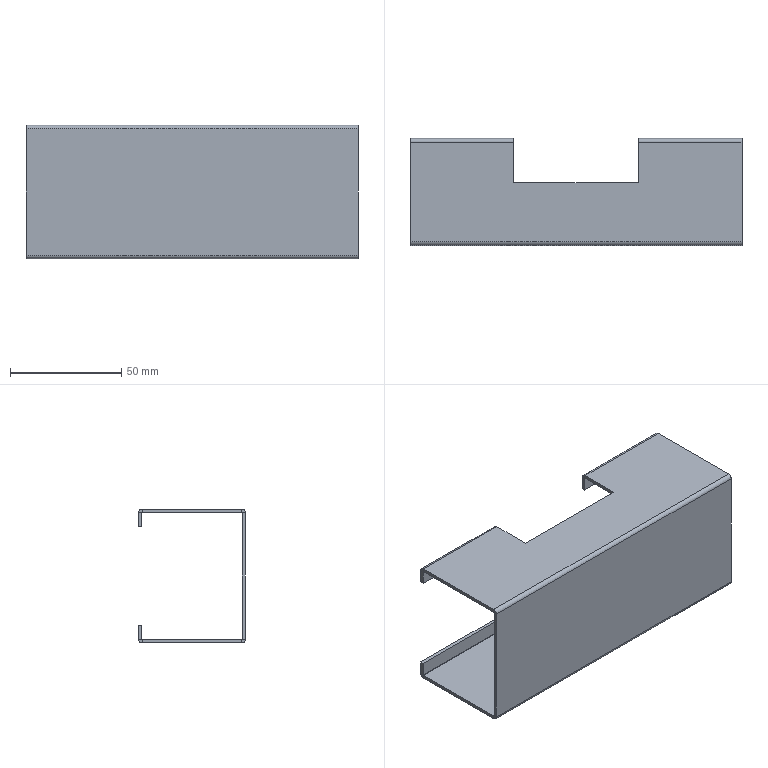Part | 1 solid | 62 faces | box 149 x 48 x 60 mm | volume 32353 mm3 | plane 50 | cylinder 12 | commonest cylinder face diameters 0.4 x6 3.4 x6
STEP:
#1=CARTESIAN_POINT('',(-28.,48.,28.3));
#2=VERTEX_POINT('',#1);
#3=CARTESIAN_POINT('',(-28.,48.,22.));
#4=VERTEX_POINT('',#3);
#5=CARTESIAN_POINT('',(-28.,48.,22.));
#6=DIRECTION('',(0.,0.,-1.));
#7=VECTOR('',#6,1000.);
#8=LINE('',#5,#7);
#9=EDGE_CURVE('',#2,#4,#8,.T.);
#10=ORIENTED_EDGE('',*,*,#9,.F.);
#11=CARTESIAN_POINT('',(-28.,46.5,28.3));
#12=VERTEX_POINT('',#11);
#13=CARTESIAN_POINT('',(-28.,48.,28.3));
#14=DIRECTION('',(0.,-1.,0.));
#15=VECTOR('',#14,1000.);
#16=LINE('',#13,#15);
#17=EDGE_CURVE('',#2,#12,#16,.T.);
#18=ORIENTED_EDGE('',*,*,#17,.T.);
#19=CARTESIAN_POINT('',(-28.,46.5,22.));
#20=VERTEX_POINT('',#19);
#21=CARTESIAN_POINT('',(-28.,46.5,22.));
#22=DIRECTION('',(0.,0.,-1.));
#23=VECTOR('',#22,1000.);
#24=LINE('',#21,#23);
#25=EDGE_CURVE('',#12,#20,#24,.T.);
#26=ORIENTED_EDGE('',*,*,#25,.T.);
#27=CARTESIAN_POINT('',(-28.,48.,22.));
#28=DIRECTION('',(0.,1.,0.));
#29=VECTOR('',#28,1000.);
#30=LINE('',#27,#29);
#31=EDGE_CURVE('',#20,#4,#30,.T.);
#32=ORIENTED_EDGE('',*,*,#31,.T.);
#33=EDGE_LOOP('',(#10,#18,#26,#32));
#34=FACE_OUTER_BOUND('',#33,.T.);
#35=CARTESIAN_POINT('',(-28.,68.,-30.));
#36=DIRECTION('',(-1.,0.,0.));
#37=DIRECTION('',(0.,0.,1.));
#38=AXIS2_PLACEMENT_3D('',#35,#36,#37);
#39=PLANE('',#38);
#40=ADVANCED_FACE('',(#34),#39,.F.);
#41=CARTESIAN_POINT('',(-28.,28.,28.5));
#42=VERTEX_POINT('',#41);
#43=CARTESIAN_POINT('',(-28.,46.3,28.5));
#44=VERTEX_POINT('',#43);
#45=CARTESIAN_POINT('',(-28.,48.,28.5));
#46=DIRECTION('',(0.,1.,0.));
#47=VECTOR('',#46,1000.);
#48=LINE('',#45,#47);
#49=EDGE_CURVE('',#42,#44,#48,.T.);
#50=ORIENTED_EDGE('',*,*,#49,.T.);
#51=CARTESIAN_POINT('',(-28.,46.3,30.));
#52=VERTEX_POINT('',#51);
#53=CARTESIAN_POINT('',(-28.,46.3,28.5));
#54=DIRECTION('',(0.,0.,1.));
#55=VECTOR('',#54,1000.);
#56=LINE('',#53,#55);
#57=EDGE_CURVE('',#44,#52,#56,.T.);
#58=ORIENTED_EDGE('',*,*,#57,.T.);
#59=CARTESIAN_POINT('',(-28.,28.,30.));
#60=VERTEX_POINT('',#59);
#61=CARTESIAN_POINT('',(-28.,48.,30.));
#62=DIRECTION('',(0.,1.,0.));
#63=VECTOR('',#62,1000.);
#64=LINE('',#61,#63);
#65=EDGE_CURVE('',#60,#52,#64,.T.);
#66=ORIENTED_EDGE('',*,*,#65,.F.);
#67=CARTESIAN_POINT('',(-28.,28.,-30.));
#68=DIRECTION('',(0.,0.,1.));
#69=VECTOR('',#68,1000.);
#70=LINE('',#67,#69);
#71=EDGE_CURVE('',#42,#60,#70,.T.);
#72=ORIENTED_EDGE('',*,*,#71,.F.);
#73=EDGE_LOOP('',(#50,#58,#66,#72));
#74=FACE_OUTER_BOUND('',#73,.T.);
#75=CARTESIAN_POINT('',(-28.,68.,-30.));
#76=DIRECTION('',(-1.,0.,0.));
#77=DIRECTION('',(0.,0.,1.));
#78=AXIS2_PLACEMENT_3D('',#75,#76,#77);
#79=PLANE('',#78);
#80=ADVANCED_FACE('',(#74),#79,.F.);
#81=CARTESIAN_POINT('',(28.,46.5,22.));
#82=VERTEX_POINT('',#81);
#83=CARTESIAN_POINT('',(28.,46.5,28.3));
#84=VERTEX_POINT('',#83);
#85=CARTESIAN_POINT('',(28.,46.5,22.));
#86=DIRECTION('',(0.,0.,1.));
#87=VECTOR('',#86,1000.);
#88=LINE('',#85,#87);
#89=EDGE_CURVE('',#82,#84,#88,.T.);
#90=ORIENTED_EDGE('',*,*,#89,.T.);
#91=CARTESIAN_POINT('',(28.,48.,28.3));
#92=VERTEX_POINT('',#91);
#93=CARTESIAN_POINT('',(28.,46.5,28.3));
#94=DIRECTION('',(0.,1.,0.));
#95=VECTOR('',#94,1000.);
#96=LINE('',#93,#95);
#97=EDGE_CURVE('',#84,#92,#96,.T.);
#98=ORIENTED_EDGE('',*,*,#97,.T.);
#99=CARTESIAN_POINT('',(28.,48.,22.));
#100=VERTEX_POINT('',#99);
#101=CARTESIAN_POINT('',(28.,48.,22.));
#102=DIRECTION('',(0.,0.,1.));
#103=VECTOR('',#102,1000.);
#104=LINE('',#101,#103);
#105=EDGE_CURVE('',#100,#92,#104,.T.);
#106=ORIENTED_EDGE('',*,*,#105,.F.);
#107=CARTESIAN_POINT('',(28.,48.,22.));
#108=DIRECTION('',(0.,-1.,0.));
#109=VECTOR('',#108,1000.);
#110=LINE('',#107,#109);
#111=EDGE_CURVE('',#100,#82,#110,.T.);
#112=ORIENTED_EDGE('',*,*,#111,.T.);
#113=EDGE_LOOP('',(#90,#98,#106,#112));
#114=FACE_OUTER_BOUND('',#113,.T.);
#115=CARTESIAN_POINT('',(28.,68.,-30.));
#116=DIRECTION('',(1.,0.,0.));
#117=DIRECTION('',(0.,0.,-1.));
#118=AXIS2_PLACEMENT_3D('',#115,#116,#117);
#119=PLANE('',#118);
#120=ADVANCED_FACE('',(#114),#119,.F.);
#121=CARTESIAN_POINT('',(28.,46.3,30.));
#122=VERTEX_POINT('',#121);
#123=CARTESIAN_POINT('',(28.,28.,30.));
#124=VERTEX_POINT('',#123);
#125=CARTESIAN_POINT('',(28.,48.,30.));
#126=DIRECTION('',(0.,-1.,0.));
#127=VECTOR('',#126,1000.);
#128=LINE('',#125,#127);
#129=EDGE_CURVE('',#122,#124,#128,.T.);
#130=ORIENTED_EDGE('',*,*,#129,.F.);
#131=CARTESIAN_POINT('',(28.,46.3,28.5));
#132=VERTEX_POINT('',#131);
#133=CARTESIAN_POINT('',(28.,46.3,30.));
#134=DIRECTION('',(0.,0.,-1.));
#135=VECTOR('',#134,1000.);
#136=LINE('',#133,#135);
#137=EDGE_CURVE('',#122,#132,#136,.T.);
#138=ORIENTED_EDGE('',*,*,#137,.T.);
#139=CARTESIAN_POINT('',(28.,28.,28.5));
#140=VERTEX_POINT('',#139);
#141=CARTESIAN_POINT('',(28.,48.,28.5));
#142=DIRECTION('',(0.,-1.,0.));
#143=VECTOR('',#142,1000.);
#144=LINE('',#141,#143);
#145=EDGE_CURVE('',#132,#140,#144,.T.);
#146=ORIENTED_EDGE('',*,*,#145,.T.);
#147=CARTESIAN_POINT('',(28.,28.,-30.));
#148=DIRECTION('',(0.,0.,1.));
#149=VECTOR('',#148,1000.);
#150=LINE('',#147,#149);
#151=EDGE_CURVE('',#140,#124,#150,.T.);
#152=ORIENTED_EDGE('',*,*,#151,.T.);
#153=EDGE_LOOP('',(#130,#138,#146,#152));
#154=FACE_OUTER_BOUND('',#153,.T.);
#155=CARTESIAN_POINT('',(28.,68.,-30.));
#156=DIRECTION('',(1.,0.,0.));
#157=DIRECTION('',(0.,0.,-1.));
#158=AXIS2_PLACEMENT_3D('',#155,#156,#157);
#159=PLANE('',#158);
#160=ADVANCED_FACE('',(#154),#159,.F.);
#161=CARTESIAN_POINT('',(-28.,46.5,-22.));
#162=VERTEX_POINT('',#161);
#163=CARTESIAN_POINT('',(-28.,46.5,-28.3));
#164=VERTEX_POINT('',#163);
#165=CARTESIAN_POINT('',(-28.,46.5,-30.));
#166=DIRECTION('',(0.,0.,-1.));
#167=VECTOR('',#166,1000.);
#168=LINE('',#165,#167);
#169=EDGE_CURVE('',#162,#164,#168,.T.);
#170=ORIENTED_EDGE('',*,*,#169,.T.);
#171=CARTESIAN_POINT('',(-28.,48.,-28.3));
#172=VERTEX_POINT('',#171);
#173=CARTESIAN_POINT('',(-28.,46.5,-28.3));
#174=DIRECTION('',(0.,1.,0.));
#175=VECTOR('',#174,1000.);
#176=LINE('',#173,#175);
#177=EDGE_CURVE('',#164,#172,#176,.T.);
#178=ORIENTED_EDGE('',*,*,#177,.T.);
#179=CARTESIAN_POINT('',(-28.,48.,-22.));
#180=VERTEX_POINT('',#179);
#181=CARTESIAN_POINT('',(-28.,48.,-30.));
#182=DIRECTION('',(0.,0.,-1.));
#183=VECTOR('',#182,1000.);
#184=LINE('',#181,#183);
#185=EDGE_CURVE('',#180,#172,#184,.T.);
#186=ORIENTED_EDGE('',*,*,#185,.F.);
#187=CARTESIAN_POINT('',(-28.,46.5,-22.));
#188=DIRECTION('',(0.,-1.,0.));
#189=VECTOR('',#188,1000.);
#190=LINE('',#187,#189);
#191=EDGE_CURVE('',#180,#162,#190,.T.);
#192=ORIENTED_EDGE('',*,*,#191,.T.);
#193=EDGE_LOOP('',(#170,#178,#186,#192));
#194=FACE_OUTER_BOUND('',#193,.T.);
#195=CARTESIAN_POINT('',(-28.,68.,-30.));
#196=DIRECTION('',(-1.,0.,0.));
#197=DIRECTION('',(0.,0.,1.));
#198=AXIS2_PLACEMENT_3D('',#195,#196,#197);
#199=PLANE('',#198);
#200=ADVANCED_FACE('',(#194),#199,.F.);
#201=CARTESIAN_POINT('',(-28.,46.3,-30.));
#202=VERTEX_POINT('',#201);
#203=CARTESIAN_POINT('',(-28.,28.,-30.));
#204=VERTEX_POINT('',#203);
#205=CARTESIAN_POINT('',(-28.,68.,-30.));
#206=DIRECTION('',(0.,-1.,0.));
#207=VECTOR('',#206,1000.);
#208=LINE('',#205,#207);
#209=EDGE_CURVE('',#202,#204,#208,.T.);
#210=ORIENTED_EDGE('',*,*,#209,.F.);
#211=CARTESIAN_POINT('',(-28.,46.3,-28.5));
#212=VERTEX_POINT('',#211);
#213=CARTESIAN_POINT('',(-28.,46.3,-30.));
#214=DIRECTION('',(0.,0.,1.));
#215=VECTOR('',#214,1000.);
#216=LINE('',#213,#215);
#217=EDGE_CURVE('',#202,#212,#216,.T.);
#218=ORIENTED_EDGE('',*,*,#217,.T.);
#219=CARTESIAN_POINT('',(-28.,28.,-28.5));
#220=VERTEX_POINT('',#219);
#221=CARTESIAN_POINT('',(-28.,0.,-28.5));
#222=DIRECTION('',(0.,-1.,0.));
#223=VECTOR('',#222,1000.);
#224=LINE('',#221,#223);
#225=EDGE_CURVE('',#212,#220,#224,.T.);
#226=ORIENTED_EDGE('',*,*,#225,.T.);
#227=CARTESIAN_POINT('',(-28.,28.,-30.));
#228=DIRECTION('',(0.,0.,1.));
#229=VECTOR('',#228,1000.);
#230=LINE('',#227,#229);
#231=EDGE_CURVE('',#204,#220,#230,.T.);
#232=ORIENTED_EDGE('',*,*,#231,.F.);
#233=EDGE_LOOP('',(#210,#218,#226,#232));
#234=FACE_OUTER_BOUND('',#233,.T.);
#235=CARTESIAN_POINT('',(-28.,68.,-30.));
#236=DIRECTION('',(-1.,0.,0.));
#237=DIRECTION('',(0.,0.,1.));
#238=AXIS2_PLACEMENT_3D('',#235,#236,#237);
#239=PLANE('',#238);
#240=ADVANCED_FACE('',(#234),#239,.F.);
#241=CARTESIAN_POINT('',(28.,48.,-28.3));
#242=VERTEX_POINT('',#241);
#243=CARTESIAN_POINT('',(28.,48.,-22.));
#244=VERTEX_POINT('',#243);
#245=CARTESIAN_POINT('',(28.,48.,-30.));
#246=DIRECTION('',(0.,0.,1.));
#247=VECTOR('',#246,1000.);
#248=LINE('',#245,#247);
#249=EDGE_CURVE('',#242,#244,#248,.T.);
#250=ORIENTED_EDGE('',*,*,#249,.F.);
#251=CARTESIAN_POINT('',(28.,46.5,-28.3));
#252=VERTEX_POINT('',#251);
#253=CARTESIAN_POINT('',(28.,48.,-28.3));
#254=DIRECTION('',(0.,-1.,0.));
#255=VECTOR('',#254,1000.);
#256=LINE('',#253,#255);
#257=EDGE_CURVE('',#242,#252,#256,.T.);
#258=ORIENTED_EDGE('',*,*,#257,.T.);
#259=CARTESIAN_POINT('',(28.,46.5,-22.));
#260=VERTEX_POINT('',#259);
#261=CARTESIAN_POINT('',(28.,46.5,-30.));
#262=DIRECTION('',(0.,0.,1.));
#263=VECTOR('',#262,1000.);
#264=LINE('',#261,#263);
#265=EDGE_CURVE('',#252,#260,#264,.T.);
#266=ORIENTED_EDGE('',*,*,#265,.T.);
#267=CARTESIAN_POINT('',(28.,46.5,-22.));
#268=DIRECTION('',(0.,1.,0.));
#269=VECTOR('',#268,1000.);
#270=LINE('',#267,#269);
#271=EDGE_CURVE('',#260,#244,#270,.T.);
#272=ORIENTED_EDGE('',*,*,#271,.T.);
#273=EDGE_LOOP('',(#250,#258,#266,#272));
#274=FACE_OUTER_BOUND('',#273,.T.);
#275=CARTESIAN_POINT('',(28.,68.,-30.));
#276=DIRECTION('',(1.,0.,0.));
#277=DIRECTION('',(0.,0.,-1.));
#278=AXIS2_PLACEMENT_3D('',#275,#276,#277);
#279=PLANE('',#278);
#280=ADVANCED_FACE('',(#274),#279,.F.);
#281=CARTESIAN_POINT('',(28.,28.,-28.5));
#282=VERTEX_POINT('',#281);
#283=CARTESIAN_POINT('',(28.,46.3,-28.5));
#284=VERTEX_POINT('',#283);
#285=CARTESIAN_POINT('',(28.,0.,-28.5));
#286=DIRECTION('',(0.,1.,0.));
#287=VECTOR('',#286,1000.);
#288=LINE('',#285,#287);
#289=EDGE_CURVE('',#282,#284,#288,.T.);
#290=ORIENTED_EDGE('',*,*,#289,.T.);
#291=CARTESIAN_POINT('',(28.,46.3,-30.));
#292=VERTEX_POINT('',#291);
#293=CARTESIAN_POINT('',(28.,46.3,-28.5));
#294=DIRECTION('',(0.,0.,-1.));
#295=VECTOR('',#294,1000.);
#296=LINE('',#293,#295);
#297=EDGE_CURVE('',#284,#292,#296,.T.);
#298=ORIENTED_EDGE('',*,*,#297,.T.);
#299=CARTESIAN_POINT('',(28.,28.,-30.));
#300=VERTEX_POINT('',#299);
#301=CARTESIAN_POINT('',(28.,68.,-30.));
#302=DIRECTION('',(0.,1.,0.));
#303=VECTOR('',#302,1000.);
#304=LINE('',#301,#303);
#305=EDGE_CURVE('',#300,#292,#304,.T.);
#306=ORIENTED_EDGE('',*,*,#305,.F.);
#307=CARTESIAN_POINT('',(28.,28.,-30.));
#308=DIRECTION('',(0.,0.,1.));
#309=VECTOR('',#308,1000.);
#310=LINE('',#307,#309);
#311=EDGE_CURVE('',#300,#282,#310,.T.);
#312=ORIENTED_EDGE('',*,*,#311,.T.);
#313=EDGE_LOOP('',(#290,#298,#306,#312));
#314=FACE_OUTER_BOUND('',#313,.T.);
#315=CARTESIAN_POINT('',(28.,68.,-30.));
#316=DIRECTION('',(1.,0.,0.));
#317=DIRECTION('',(0.,0.,-1.));
#318=AXIS2_PLACEMENT_3D('',#315,#316,#317);
#319=PLANE('',#318);
#320=ADVANCED_FACE('',(#314),#319,.F.);
#321=CARTESIAN_POINT('',(74.5,48.,-28.3));
#322=VERTEX_POINT('',#321);
#323=CARTESIAN_POINT('',(74.5,48.,-28.3));
#324=DIRECTION('',(-1.,0.,0.));
#325=VECTOR('',#324,1000.);
#326=LINE('',#323,#325);
#327=EDGE_CURVE('',#322,#242,#326,.T.);
#328=ORIENTED_EDGE('',*,*,#327,.T.);
#329=ORIENTED_EDGE('',*,*,#249,.T.);
#330=CARTESIAN_POINT('',(74.5,48.,-22.));
#331=VERTEX_POINT('',#330);
#332=CARTESIAN_POINT('',(74.5,48.,-22.));
#333=DIRECTION('',(-1.,0.,0.));
#334=VECTOR('',#333,1000.);
#335=LINE('',#332,#334);
#336=EDGE_CURVE('',#331,#244,#335,.T.);
#337=ORIENTED_EDGE('',*,*,#336,.F.);
#338=CARTESIAN_POINT('',(74.5,48.,-30.));
#339=DIRECTION('',(0.,0.,1.));
#340=VECTOR('',#339,1000.);
#341=LINE('',#338,#340);
#342=EDGE_CURVE('',#322,#331,#341,.T.);
#343=ORIENTED_EDGE('',*,*,#342,.F.);
#344=EDGE_LOOP('',(#328,#329,#337,#343));
#345=FACE_OUTER_BOUND('',#344,.T.);
#346=CARTESIAN_POINT('',(74.5,48.,-30.));
#347=DIRECTION('',(0.,-1.,0.));
#348=DIRECTION('',(0.,0.,-1.));
#349=AXIS2_PLACEMENT_3D('',#346,#347,#348);
#350=PLANE('',#349);
#351=ADVANCED_FACE('',(#345),#350,.F.);
#352=ORIENTED_EDGE('',*,*,#271,.F.);
#353=CARTESIAN_POINT('',(74.5,46.5,-22.));
#354=VERTEX_POINT('',#353);
#355=CARTESIAN_POINT('',(74.5,46.5,-22.));
#356=DIRECTION('',(-1.,0.,0.));
#357=VECTOR('',#356,1000.);
#358=LINE('',#355,#357);
#359=EDGE_CURVE('',#354,#260,#358,.T.);
#360=ORIENTED_EDGE('',*,*,#359,.F.);
#361=CARTESIAN_POINT('',(74.5,46.5,-22.));
#362=DIRECTION('',(0.,1.,0.));
#363=VECTOR('',#362,1000.);
#364=LINE('',#361,#363);
#365=EDGE_CURVE('',#354,#331,#364,.T.);
#366=ORIENTED_EDGE('',*,*,#365,.T.);
#367=ORIENTED_EDGE('',*,*,#336,.T.);
#368=EDGE_LOOP('',(#352,#360,#366,#367));
#369=FACE_OUTER_BOUND('',#368,.T.);
#370=CARTESIAN_POINT('',(74.5,46.5,-22.));
#371=DIRECTION('',(0.,0.,1.));
#372=DIRECTION('',(1.,0.,0.));
#373=AXIS2_PLACEMENT_3D('',#370,#371,#372);
#374=PLANE('',#373);
#375=ADVANCED_FACE('',(#369),#374,.T.);
#376=ORIENTED_EDGE('',*,*,#265,.F.);
#377=CARTESIAN_POINT('',(74.5,46.5,-28.3));
#378=VERTEX_POINT('',#377);
#379=CARTESIAN_POINT('',(74.5,46.5,-28.3));
#380=DIRECTION('',(-1.,0.,0.));
#381=VECTOR('',#380,1000.);
#382=LINE('',#379,#381);
#383=EDGE_CURVE('',#378,#252,#382,.T.);
#384=ORIENTED_EDGE('',*,*,#383,.F.);
#385=CARTESIAN_POINT('',(74.5,46.5,-30.));
#386=DIRECTION('',(0.,0.,1.));
#387=VECTOR('',#386,1000.);
#388=LINE('',#385,#387);
#389=EDGE_CURVE('',#378,#354,#388,.T.);
#390=ORIENTED_EDGE('',*,*,#389,.T.);
#391=ORIENTED_EDGE('',*,*,#359,.T.);
#392=EDGE_LOOP('',(#376,#384,#390,#391));
#393=FACE_OUTER_BOUND('',#392,.T.);
#394=CARTESIAN_POINT('',(74.5,46.5,-30.));
#395=DIRECTION('',(0.,-1.,0.));
#396=DIRECTION('',(0.,0.,-1.));
#397=AXIS2_PLACEMENT_3D('',#394,#395,#396);
#398=PLANE('',#397);
#399=ADVANCED_FACE('',(#393),#398,.T.);
#400=CARTESIAN_POINT('',(28.,46.3,-28.3));
#401=DIRECTION('',(1.,0.,0.));
#402=DIRECTION('',(0.,0.,-1.));
#403=AXIS2_PLACEMENT_3D('',#400,#401,#402);
#404=CIRCLE('',#403,0.2);
#405=EDGE_CURVE('',#284,#252,#404,.T.);
#406=ORIENTED_EDGE('',*,*,#405,.F.);
#407=CARTESIAN_POINT('',(74.5,46.3,-28.5));
#408=VERTEX_POINT('',#407);
#409=CARTESIAN_POINT('',(74.5,46.3,-28.5));
#410=DIRECTION('',(-1.,0.,0.));
#411=VECTOR('',#410,1000.);
#412=LINE('',#409,#411);
#413=EDGE_CURVE('',#408,#284,#412,.T.);
#414=ORIENTED_EDGE('',*,*,#413,.F.);
#415=CARTESIAN_POINT('',(74.5,46.3,-28.3));
#416=DIRECTION('',(1.,0.,0.));
#417=DIRECTION('',(0.,0.,-1.));
#418=AXIS2_PLACEMENT_3D('',#415,#416,#417);
#419=CIRCLE('',#418,0.2);
#420=EDGE_CURVE('',#408,#378,#419,.T.);
#421=ORIENTED_EDGE('',*,*,#420,.T.);
#422=ORIENTED_EDGE('',*,*,#383,.T.);
#423=EDGE_LOOP('',(#406,#414,#421,#422));
#424=FACE_OUTER_BOUND('',#423,.T.);
#425=CARTESIAN_POINT('',(74.5,46.3,-28.3));
#426=DIRECTION('',(-1.,0.,0.));
#427=DIRECTION('',(0.,0.,1.));
#428=AXIS2_PLACEMENT_3D('',#425,#426,#427);
#429=CYLINDRICAL_SURFACE('',#428,0.2);
#430=ADVANCED_FACE('',(#424),#429,.F.);
#431=CARTESIAN_POINT('',(28.,46.3,28.3));
#432=DIRECTION('',(1.,0.,0.));
#433=DIRECTION('',(0.,0.,-1.));
#434=AXIS2_PLACEMENT_3D('',#431,#432,#433);
#435=CIRCLE('',#434,0.2);
#436=EDGE_CURVE('',#84,#132,#435,.T.);
#437=ORIENTED_EDGE('',*,*,#436,.F.);
#438=CARTESIAN_POINT('',(74.5,46.5,28.3));
#439=VERTEX_POINT('',#438);
#440=CARTESIAN_POINT('',(74.5,46.5,28.3));
#441=DIRECTION('',(-1.,0.,0.));
#442=VECTOR('',#441,1000.);
#443=LINE('',#440,#442);
#444=EDGE_CURVE('',#439,#84,#443,.T.);
#445=ORIENTED_EDGE('',*,*,#444,.F.);
#446=CARTESIAN_POINT('',(74.5,46.3,28.5));
#447=VERTEX_POINT('',#446);
#448=CARTESIAN_POINT('',(74.5,46.3,28.3));
#449=DIRECTION('',(1.,0.,0.));
#450=DIRECTION('',(0.,0.,-1.));
#451=AXIS2_PLACEMENT_3D('',#448,#449,#450);
#452=CIRCLE('',#451,0.2);
#453=EDGE_CURVE('',#439,#447,#452,.T.);
#454=ORIENTED_EDGE('',*,*,#453,.T.);
#455=CARTESIAN_POINT('',(74.5,46.3,28.5));
#456=DIRECTION('',(-1.,0.,0.));
#457=VECTOR('',#456,1000.);
#458=LINE('',#455,#457);
#459=EDGE_CURVE('',#447,#132,#458,.T.);
#460=ORIENTED_EDGE('',*,*,#459,.T.);
#461=EDGE_LOOP('',(#437,#445,#454,#460));
#462=FACE_OUTER_BOUND('',#461,.T.);
#463=CARTESIAN_POINT('',(74.5,46.3,28.3));
#464=DIRECTION('',(-1.,0.,0.));
#465=DIRECTION('',(0.,0.,1.));
#466=AXIS2_PLACEMENT_3D('',#463,#464,#465);
#467=CYLINDRICAL_SURFACE('',#466,0.2);
#468=ADVANCED_FACE('',(#462),#467,.F.);
#469=ORIENTED_EDGE('',*,*,#89,.F.);
#470=CARTESIAN_POINT('',(74.5,46.5,22.));
#471=VERTEX_POINT('',#470);
#472=CARTESIAN_POINT('',(74.5,46.5,22.));
#473=DIRECTION('',(-1.,0.,0.));
#474=VECTOR('',#473,1000.);
#475=LINE('',#472,#474);
#476=EDGE_CURVE('',#471,#82,#475,.T.);
#477=ORIENTED_EDGE('',*,*,#476,.F.);
#478=CARTESIAN_POINT('',(74.5,46.5,22.));
#479=DIRECTION('',(0.,0.,1.));
#480=VECTOR('',#479,1000.);
#481=LINE('',#478,#480);
#482=EDGE_CURVE('',#471,#439,#481,.T.);
#483=ORIENTED_EDGE('',*,*,#482,.T.);
#484=ORIENTED_EDGE('',*,*,#444,.T.);
#485=EDGE_LOOP('',(#469,#477,#483,#484));
#486=FACE_OUTER_BOUND('',#485,.T.);
#487=CARTESIAN_POINT('',(74.5,46.5,22.));
#488=DIRECTION('',(0.,-1.,0.));
#489=DIRECTION('',(0.,0.,-1.));
#490=AXIS2_PLACEMENT_3D('',#487,#488,#489);
#491=PLANE('',#490);
#492=ADVANCED_FACE('',(#486),#491,.T.);
#493=ORIENTED_EDGE('',*,*,#111,.F.);
#494=CARTESIAN_POINT('',(74.5,48.,22.));
#495=VERTEX_POINT('',#494);
#496=CARTESIAN_POINT('',(74.5,48.,22.));
#497=DIRECTION('',(-1.,0.,0.));
#498=VECTOR('',#497,1000.);
#499=LINE('',#496,#498);
#500=EDGE_CURVE('',#495,#100,#499,.T.);
#501=ORIENTED_EDGE('',*,*,#500,.F.);
#502=CARTESIAN_POINT('',(74.5,48.,22.));
#503=DIRECTION('',(0.,-1.,0.));
#504=VECTOR('',#503,1000.);
#505=LINE('',#502,#504);
#506=EDGE_CURVE('',#495,#471,#505,.T.);
#507=ORIENTED_EDGE('',*,*,#506,.T.);
#508=ORIENTED_EDGE('',*,*,#476,.T.);
#509=EDGE_LOOP('',(#493,#501,#507,#508));
#510=FACE_OUTER_BOUND('',#509,.T.);
#511=CARTESIAN_POINT('',(74.5,48.,22.));
#512=DIRECTION('',(0.,0.,-1.));
#513=DIRECTION('',(-1.,0.,0.));
#514=AXIS2_PLACEMENT_3D('',#511,#512,#513);
#515=PLANE('',#514);
#516=ADVANCED_FACE('',(#510),#515,.T.);
#517=ORIENTED_EDGE('',*,*,#500,.T.);
#518=ORIENTED_EDGE('',*,*,#105,.T.);
#519=CARTESIAN_POINT('',(74.5,48.,28.3));
#520=VERTEX_POINT('',#519);
#521=CARTESIAN_POINT('',(74.5,48.,28.3));
#522=DIRECTION('',(-1.,0.,0.));
#523=VECTOR('',#522,1000.);
#524=LINE('',#521,#523);
#525=EDGE_CURVE('',#520,#92,#524,.T.);
#526=ORIENTED_EDGE('',*,*,#525,.F.);
#527=CARTESIAN_POINT('',(74.5,48.,22.));
#528=DIRECTION('',(0.,0.,1.));
#529=VECTOR('',#528,1000.);
#530=LINE('',#527,#529);
#531=EDGE_CURVE('',#495,#520,#530,.T.);
#532=ORIENTED_EDGE('',*,*,#531,.F.);
#533=EDGE_LOOP('',(#517,#518,#526,#532));
#534=FACE_OUTER_BOUND('',#533,.T.);
#535=CARTESIAN_POINT('',(74.5,48.,22.));
#536=DIRECTION('',(0.,-1.,0.));
#537=DIRECTION('',(0.,0.,-1.));
#538=AXIS2_PLACEMENT_3D('',#535,#536,#537);
#539=PLANE('',#538);
#540=ADVANCED_FACE('',(#534),#539,.F.);
#541=ORIENTED_EDGE('',*,*,#525,.T.);
#542=CARTESIAN_POINT('',(28.,46.3,28.3));
#543=DIRECTION('',(1.,0.,0.));
#544=DIRECTION('',(0.,0.,-1.));
#545=AXIS2_PLACEMENT_3D('',#542,#543,#544);
#546=CIRCLE('',#545,1.7);
#547=EDGE_CURVE('',#92,#122,#546,.T.);
#548=ORIENTED_EDGE('',*,*,#547,.T.);
#549=CARTESIAN_POINT('',(74.5,46.3,30.));
#550=VERTEX_POINT('',#549);
#551=CARTESIAN_POINT('',(74.5,46.3,30.));
#552=DIRECTION('',(-1.,0.,0.));
#553=VECTOR('',#552,1000.);
#554=LINE('',#551,#553);
#555=EDGE_CURVE('',#550,#122,#554,.T.);
#556=ORIENTED_EDGE('',*,*,#555,.F.);
#557=CARTESIAN_POINT('',(74.5,46.3,28.3));
#558=DIRECTION('',(1.,0.,0.));
#559=DIRECTION('',(0.,0.,1.));
#560=AXIS2_PLACEMENT_3D('',#557,#558,#559);
#561=CIRCLE('',#560,1.7);
#562=EDGE_CURVE('',#520,#550,#561,.T.);
#563=ORIENTED_EDGE('',*,*,#562,.F.);
#564=EDGE_LOOP('',(#541,#548,#556,#563));
#565=FACE_OUTER_BOUND('',#564,.T.);
#566=CARTESIAN_POINT('',(74.5,46.3,28.3));
#567=DIRECTION('',(-1.,0.,0.));
#568=DIRECTION('',(0.,0.,1.));
#569=AXIS2_PLACEMENT_3D('',#566,#567,#568);
#570=CYLINDRICAL_SURFACE('',#569,1.7);
#571=ADVANCED_FACE('',(#565),#570,.T.);
#572=CARTESIAN_POINT('',(74.5,46.3,-30.));
#573=VERTEX_POINT('',#572);
#574=CARTESIAN_POINT('',(74.5,46.3,-30.));
#575=DIRECTION('',(-1.,0.,0.));
#576=VECTOR('',#575,1000.);
#577=LINE('',#574,#576);
#578=EDGE_CURVE('',#573,#292,#577,.T.);
#579=ORIENTED_EDGE('',*,*,#578,.T.);
#580=CARTESIAN_POINT('',(28.,46.3,-28.3));
#581=DIRECTION('',(1.,0.,0.));
#582=DIRECTION('',(0.,0.,-1.));
#583=AXIS2_PLACEMENT_3D('',#580,#581,#582);
#584=CIRCLE('',#583,1.7);
#585=EDGE_CURVE('',#292,#242,#584,.T.);
#586=ORIENTED_EDGE('',*,*,#585,.T.);
#587=ORIENTED_EDGE('',*,*,#327,.F.);
#588=CARTESIAN_POINT('',(74.5,46.3,-28.3));
#589=DIRECTION('',(1.,0.,0.));
#590=DIRECTION('',(0.,0.,1.));
#591=AXIS2_PLACEMENT_3D('',#588,#589,#590);
#592=CIRCLE('',#591,1.7);
#593=EDGE_CURVE('',#573,#322,#592,.T.);
#594=ORIENTED_EDGE('',*,*,#593,.F.);
#595=EDGE_LOOP('',(#579,#586,#587,#594));
#596=FACE_OUTER_BOUND('',#595,.T.);
#597=CARTESIAN_POINT('',(74.5,46.3,-28.3));
#598=DIRECTION('',(-1.,0.,0.));
#599=DIRECTION('',(0.,0.,1.));
#600=AXIS2_PLACEMENT_3D('',#597,#598,#599);
#601=CYLINDRICAL_SURFACE('',#600,1.7);
#602=ADVANCED_FACE('',(#596),#601,.T.);
#603=CARTESIAN_POINT('',(74.5,48.,28.3));
#604=DIRECTION('',(0.,-1.,0.));
#605=VECTOR('',#604,1000.);
#606=LINE('',#603,#605);
#607=EDGE_CURVE('',#520,#439,#606,.T.);
#608=ORIENTED_EDGE('',*,*,#607,.F.);
#609=ORIENTED_EDGE('',*,*,#562,.T.);
#610=CARTESIAN_POINT('',(74.5,46.3,28.5));
#611=DIRECTION('',(0.,0.,1.));
#612=VECTOR('',#611,1000.);
#613=LINE('',#610,#612);
#614=EDGE_CURVE('',#447,#550,#613,.T.);
#615=ORIENTED_EDGE('',*,*,#614,.F.);
#616=ORIENTED_EDGE('',*,*,#453,.F.);
#617=EDGE_LOOP('',(#608,#609,#615,#616));
#618=FACE_OUTER_BOUND('',#617,.T.);
#619=CARTESIAN_POINT('',(74.5,48.,28.3));
#620=DIRECTION('',(1.,0.,0.));
#621=DIRECTION('',(0.,0.,-1.));
#622=AXIS2_PLACEMENT_3D('',#619,#620,#621);
#623=PLANE('',#622);
#624=ADVANCED_FACE('',(#618),#623,.T.);
#625=ORIENTED_EDGE('',*,*,#531,.T.);
#626=ORIENTED_EDGE('',*,*,#607,.T.);
#627=ORIENTED_EDGE('',*,*,#482,.F.);
#628=ORIENTED_EDGE('',*,*,#506,.F.);
#629=EDGE_LOOP('',(#625,#626,#627,#628));
#630=FACE_OUTER_BOUND('',#629,.T.);
#631=CARTESIAN_POINT('',(74.5,46.3,28.5));
#632=DIRECTION('',(1.,0.,0.));
#633=DIRECTION('',(0.,0.,-1.));
#634=AXIS2_PLACEMENT_3D('',#631,#632,#633);
#635=PLANE('',#634);
#636=ADVANCED_FACE('',(#630),#635,.T.);
#637=CARTESIAN_POINT('',(-74.5,46.3,30.));
#638=VERTEX_POINT('',#637);
#639=CARTESIAN_POINT('',(-74.5,46.3,28.5));
#640=VERTEX_POINT('',#639);
#641=CARTESIAN_POINT('',(-74.5,46.3,30.));
#642=DIRECTION('',(0.,0.,-1.));
#643=VECTOR('',#642,1000.);
#644=LINE('',#641,#643);
#645=EDGE_CURVE('',#638,#640,#644,.T.);
#646=ORIENTED_EDGE('',*,*,#645,.F.);
#647=CARTESIAN_POINT('',(-74.5,48.,28.3));
#648=VERTEX_POINT('',#647);
#649=CARTESIAN_POINT('',(-74.5,46.3,28.3));
#650=DIRECTION('',(1.,0.,0.));
#651=DIRECTION('',(0.,0.,1.));
#652=AXIS2_PLACEMENT_3D('',#649,#650,#651);
#653=CIRCLE('',#652,1.7);
#654=EDGE_CURVE('',#648,#638,#653,.T.);
#655=ORIENTED_EDGE('',*,*,#654,.F.);
#656=CARTESIAN_POINT('',(-74.5,46.5,28.3));
#657=VERTEX_POINT('',#656);
#658=CARTESIAN_POINT('',(-74.5,46.5,28.3));
#659=DIRECTION('',(0.,1.,0.));
#660=VECTOR('',#659,1000.);
#661=LINE('',#658,#660);
#662=EDGE_CURVE('',#657,#648,#661,.T.);
#663=ORIENTED_EDGE('',*,*,#662,.F.);
#664=CARTESIAN_POINT('',(-74.5,46.3,28.3));
#665=DIRECTION('',(1.,0.,0.));
#666=DIRECTION('',(0.,0.,-1.));
#667=AXIS2_PLACEMENT_3D('',#664,#665,#666);
#668=CIRCLE('',#667,0.2);
#669=EDGE_CURVE('',#657,#640,#668,.T.);
#670=ORIENTED_EDGE('',*,*,#669,.T.);
#671=EDGE_LOOP('',(#646,#655,#663,#670));
#672=FACE_OUTER_BOUND('',#671,.T.);
#673=CARTESIAN_POINT('',(-74.5,46.3,30.));
#674=DIRECTION('',(-1.,0.,0.));
#675=DIRECTION('',(0.,0.,1.));
#676=AXIS2_PLACEMENT_3D('',#673,#674,#675);
#677=PLANE('',#676);
#678=ADVANCED_FACE('',(#672),#677,.T.);
#679=CARTESIAN_POINT('',(-74.5,1.7,30.));
#680=VERTEX_POINT('',#679);
#681=CARTESIAN_POINT('',(-74.5,48.,30.));
#682=DIRECTION('',(0.,-1.,0.));
#683=VECTOR('',#682,1000.);
#684=LINE('',#681,#683);
#685=EDGE_CURVE('',#638,#680,#684,.T.);
#686=ORIENTED_EDGE('',*,*,#685,.F.);
#687=ORIENTED_EDGE('',*,*,#645,.T.);
#688=CARTESIAN_POINT('',(-74.5,1.7,28.5));
#689=VERTEX_POINT('',#688);
#690=CARTESIAN_POINT('',(-74.5,48.,28.5));
#691=DIRECTION('',(0.,-1.,0.));
#692=VECTOR('',#691,1000.);
#693=LINE('',#690,#692);
#694=EDGE_CURVE('',#640,#689,#693,.T.);
#695=ORIENTED_EDGE('',*,*,#694,.T.);
#696=CARTESIAN_POINT('',(-74.5,1.7,28.5));
#697=DIRECTION('',(0.,0.,1.));
#698=VECTOR('',#697,1000.);
#699=LINE('',#696,#698);
#700=EDGE_CURVE('',#689,#680,#699,.T.);
#701=ORIENTED_EDGE('',*,*,#700,.T.);
#702=EDGE_LOOP('',(#686,#687,#695,#701));
#703=FACE_OUTER_BOUND('',#702,.T.);
#704=CARTESIAN_POINT('',(-74.5,46.5,28.3));
#705=DIRECTION('',(-1.,0.,0.));
#706=DIRECTION('',(0.,0.,1.));
#707=AXIS2_PLACEMENT_3D('',#704,#705,#706);
#708=PLANE('',#707);
#709=ADVANCED_FACE('',(#703),#708,.T.);
#710=CARTESIAN_POINT('',(74.5,1.7,30.));
#711=VERTEX_POINT('',#710);
#712=CARTESIAN_POINT('',(74.5,1.7,28.5));
#713=VERTEX_POINT('',#712);
#714=CARTESIAN_POINT('',(74.5,1.7,30.));
#715=DIRECTION('',(0.,0.,-1.));
#716=VECTOR('',#715,1000.);
#717=LINE('',#714,#716);
#718=EDGE_CURVE('',#711,#713,#717,.T.);
#719=ORIENTED_EDGE('',*,*,#718,.F.);
#720=CARTESIAN_POINT('',(74.5,0.,28.3));
#721=VERTEX_POINT('',#720);
#722=CARTESIAN_POINT('',(74.5,1.7,28.3));
#723=DIRECTION('',(1.,0.,0.));
#724=DIRECTION('',(0.,0.,1.));
#725=AXIS2_PLACEMENT_3D('',#722,#723,#724);
#726=CIRCLE('',#725,1.7);
#727=EDGE_CURVE('',#711,#721,#726,.T.);
#728=ORIENTED_EDGE('',*,*,#727,.T.);
#729=CARTESIAN_POINT('',(74.5,1.5,28.3));
#730=VERTEX_POINT('',#729);
#731=CARTESIAN_POINT('',(74.5,1.5,28.3));
#732=DIRECTION('',(0.,-1.,0.));
#733=VECTOR('',#732,1000.);
#734=LINE('',#731,#733);
#735=EDGE_CURVE('',#730,#721,#734,.T.);
#736=ORIENTED_EDGE('',*,*,#735,.F.);
#737=CARTESIAN_POINT('',(74.5,1.7,28.3));
#738=DIRECTION('',(1.,0.,0.));
#739=DIRECTION('',(0.,0.,-1.));
#740=AXIS2_PLACEMENT_3D('',#737,#738,#739);
#741=CIRCLE('',#740,0.2);
#742=EDGE_CURVE('',#713,#730,#741,.T.);
#743=ORIENTED_EDGE('',*,*,#742,.F.);
#744=EDGE_LOOP('',(#719,#728,#736,#743));
#745=FACE_OUTER_BOUND('',#744,.T.);
#746=CARTESIAN_POINT('',(74.5,1.7,30.));
#747=DIRECTION('',(1.,0.,0.));
#748=DIRECTION('',(0.,0.,-1.));
#749=AXIS2_PLACEMENT_3D('',#746,#747,#748);
#750=PLANE('',#749);
#751=ADVANCED_FACE('',(#745),#750,.T.);
#752=CARTESIAN_POINT('',(74.5,48.,30.));
#753=DIRECTION('',(0.,-1.,0.));
#754=VECTOR('',#753,1000.);
#755=LINE('',#752,#754);
#756=EDGE_CURVE('',#550,#711,#755,.T.);
#757=ORIENTED_EDGE('',*,*,#756,.T.);
#758=ORIENTED_EDGE('',*,*,#718,.T.);
#759=CARTESIAN_POINT('',(74.5,48.,28.5));
#760=DIRECTION('',(0.,-1.,0.));
#761=VECTOR('',#760,1000.);
#762=LINE('',#759,#761);
#763=EDGE_CURVE('',#447,#713,#762,.T.);
#764=ORIENTED_EDGE('',*,*,#763,.F.);
#765=ORIENTED_EDGE('',*,*,#614,.T.);
#766=EDGE_LOOP('',(#757,#758,#764,#765));
#767=FACE_OUTER_BOUND('',#766,.T.);
#768=CARTESIAN_POINT('',(74.5,1.5,28.3));
#769=DIRECTION('',(1.,0.,0.));
#770=DIRECTION('',(0.,0.,-1.));
#771=AXIS2_PLACEMENT_3D('',#768,#769,#770);
#772=PLANE('',#771);
#773=ADVANCED_FACE('',(#767),#772,.T.);
#774=CARTESIAN_POINT('',(-74.5,0.,28.3));
#775=VERTEX_POINT('',#774);
#776=CARTESIAN_POINT('',(-74.5,1.5,28.3));
#777=VERTEX_POINT('',#776);
#778=CARTESIAN_POINT('',(-74.5,0.,28.3));
#779=DIRECTION('',(0.,1.,0.));
#780=VECTOR('',#779,1000.);
#781=LINE('',#778,#780);
#782=EDGE_CURVE('',#775,#777,#781,.T.);
#783=ORIENTED_EDGE('',*,*,#782,.F.);
#784=CARTESIAN_POINT('',(-74.5,1.7,28.3));
#785=DIRECTION('',(1.,0.,0.));
#786=DIRECTION('',(0.,0.,1.));
#787=AXIS2_PLACEMENT_3D('',#784,#785,#786);
#788=CIRCLE('',#787,1.7);
#789=EDGE_CURVE('',#680,#775,#788,.T.);
#790=ORIENTED_EDGE('',*,*,#789,.F.);
#791=ORIENTED_EDGE('',*,*,#700,.F.);
#792=CARTESIAN_POINT('',(-74.5,1.7,28.3));
#793=DIRECTION('',(1.,0.,0.));
#794=DIRECTION('',(0.,0.,-1.));
#795=AXIS2_PLACEMENT_3D('',#792,#793,#794);
#796=CIRCLE('',#795,0.2);
#797=EDGE_CURVE('',#689,#777,#796,.T.);
#798=ORIENTED_EDGE('',*,*,#797,.T.);
#799=EDGE_LOOP('',(#783,#790,#791,#798));
#800=FACE_OUTER_BOUND('',#799,.T.);
#801=CARTESIAN_POINT('',(-74.5,0.,28.3));
#802=DIRECTION('',(-1.,0.,0.));
#803=DIRECTION('',(0.,0.,1.));
#804=AXIS2_PLACEMENT_3D('',#801,#802,#803);
#805=PLANE('',#804);
#806=ADVANCED_FACE('',(#800),#805,.T.);
#807=CARTESIAN_POINT('',(-74.5,0.,-28.3));
#808=VERTEX_POINT('',#807);
#809=CARTESIAN_POINT('',(-74.5,0.,30.));
#810=DIRECTION('',(0.,0.,-1.));
#811=VECTOR('',#810,1000.);
#812=LINE('',#809,#811);
#813=EDGE_CURVE('',#775,#808,#812,.T.);
#814=ORIENTED_EDGE('',*,*,#813,.F.);
#815=ORIENTED_EDGE('',*,*,#782,.T.);
#816=CARTESIAN_POINT('',(-74.5,1.5,-28.3));
#817=VERTEX_POINT('',#816);
#818=CARTESIAN_POINT('',(-74.5,1.5,30.));
#819=DIRECTION('',(0.,0.,-1.));
#820=VECTOR('',#819,1000.);
#821=LINE('',#818,#820);
#822=EDGE_CURVE('',#777,#817,#821,.T.);
#823=ORIENTED_EDGE('',*,*,#822,.T.);
#824=CARTESIAN_POINT('',(-74.5,1.5,-28.3));
#825=DIRECTION('',(0.,-1.,0.));
#826=VECTOR('',#825,1000.);
#827=LINE('',#824,#826);
#828=EDGE_CURVE('',#817,#808,#827,.T.);
#829=ORIENTED_EDGE('',*,*,#828,.T.);
#830=EDGE_LOOP('',(#814,#815,#823,#829));
#831=FACE_OUTER_BOUND('',#830,.T.);
#832=CARTESIAN_POINT('',(-74.5,1.7,28.5));
#833=DIRECTION('',(-1.,0.,0.));
#834=DIRECTION('',(0.,0.,1.));
#835=AXIS2_PLACEMENT_3D('',#832,#833,#834);
#836=PLANE('',#835);
#837=ADVANCED_FACE('',(#831),#836,.T.);
#838=CARTESIAN_POINT('',(74.5,0.,-28.3));
#839=VERTEX_POINT('',#838);
#840=CARTESIAN_POINT('',(74.5,1.5,-28.3));
#841=VERTEX_POINT('',#840);
#842=CARTESIAN_POINT('',(74.5,0.,-28.3));
#843=DIRECTION('',(0.,1.,0.));
#844=VECTOR('',#843,1000.);
#845=LINE('',#842,#844);
#846=EDGE_CURVE('',#839,#841,#845,.T.);
#847=ORIENTED_EDGE('',*,*,#846,.F.);
#848=CARTESIAN_POINT('',(74.5,1.7,-30.));
#849=VERTEX_POINT('',#848);
#850=CARTESIAN_POINT('',(74.5,1.7,-28.3));
#851=DIRECTION('',(1.,0.,0.));
#852=DIRECTION('',(0.,0.,1.));
#853=AXIS2_PLACEMENT_3D('',#850,#851,#852);
#854=CIRCLE('',#853,1.7);
#855=EDGE_CURVE('',#839,#849,#854,.T.);
#856=ORIENTED_EDGE('',*,*,#855,.T.);
#857=CARTESIAN_POINT('',(74.5,1.7,-28.5));
#858=VERTEX_POINT('',#857);
#859=CARTESIAN_POINT('',(74.5,1.7,-28.5));
#860=DIRECTION('',(0.,0.,-1.));
#861=VECTOR('',#860,1000.);
#862=LINE('',#859,#861);
#863=EDGE_CURVE('',#858,#849,#862,.T.);
#864=ORIENTED_EDGE('',*,*,#863,.F.);
#865=CARTESIAN_POINT('',(74.5,1.7,-28.3));
#866=DIRECTION('',(1.,0.,0.));
#867=DIRECTION('',(0.,0.,-1.));
#868=AXIS2_PLACEMENT_3D('',#865,#866,#867);
#869=CIRCLE('',#868,0.2);
#870=EDGE_CURVE('',#841,#858,#869,.T.);
#871=ORIENTED_EDGE('',*,*,#870,.F.);
#872=EDGE_LOOP('',(#847,#856,#864,#871));
#873=FACE_OUTER_BOUND('',#872,.T.);
#874=CARTESIAN_POINT('',(74.5,0.,-28.3));
#875=DIRECTION('',(1.,0.,0.));
#876=DIRECTION('',(0.,0.,-1.));
#877=AXIS2_PLACEMENT_3D('',#874,#875,#876);
#878=PLANE('',#877);
#879=ADVANCED_FACE('',(#873),#878,.T.);
#880=CARTESIAN_POINT('',(74.5,0.,30.));
#881=DIRECTION('',(0.,0.,-1.));
#882=VECTOR('',#881,1000.);
#883=LINE('',#880,#882);
#884=EDGE_CURVE('',#721,#839,#883,.T.);
#885=ORIENTED_EDGE('',*,*,#884,.T.);
#886=ORIENTED_EDGE('',*,*,#846,.T.);
#887=CARTESIAN_POINT('',(74.5,1.5,30.));
#888=DIRECTION('',(0.,0.,-1.));
#889=VECTOR('',#888,1000.);
#890=LINE('',#887,#889);
#891=EDGE_CURVE('',#730,#841,#890,.T.);
#892=ORIENTED_EDGE('',*,*,#891,.F.);
#893=ORIENTED_EDGE('',*,*,#735,.T.);
#894=EDGE_LOOP('',(#885,#886,#892,#893));
#895=FACE_OUTER_BOUND('',#894,.T.);
#896=CARTESIAN_POINT('',(74.5,1.7,-28.5));
#897=DIRECTION('',(1.,0.,0.));
#898=DIRECTION('',(0.,0.,-1.));
#899=AXIS2_PLACEMENT_3D('',#896,#897,#898);
#900=PLANE('',#899);
#901=ADVANCED_FACE('',(#895),#900,.T.);
#902=CARTESIAN_POINT('',(-74.5,1.7,-30.));
#903=VERTEX_POINT('',#902);
#904=CARTESIAN_POINT('',(-74.5,1.7,-28.5));
#905=VERTEX_POINT('',#904);
#906=CARTESIAN_POINT('',(-74.5,1.7,-30.));
#907=DIRECTION('',(0.,0.,1.));
#908=VECTOR('',#907,1000.);
#909=LINE('',#906,#908);
#910=EDGE_CURVE('',#903,#905,#909,.T.);
#911=ORIENTED_EDGE('',*,*,#910,.F.);
#912=CARTESIAN_POINT('',(-74.5,1.7,-28.3));
#913=DIRECTION('',(1.,0.,0.));
#914=DIRECTION('',(0.,0.,1.));
#915=AXIS2_PLACEMENT_3D('',#912,#913,#914);
#916=CIRCLE('',#915,1.7);
#917=EDGE_CURVE('',#808,#903,#916,.T.);
#918=ORIENTED_EDGE('',*,*,#917,.F.);
#919=ORIENTED_EDGE('',*,*,#828,.F.);
#920=CARTESIAN_POINT('',(-74.5,1.7,-28.3));
#921=DIRECTION('',(1.,0.,0.));
#922=DIRECTION('',(0.,0.,-1.));
#923=AXIS2_PLACEMENT_3D('',#920,#921,#922);
#924=CIRCLE('',#923,0.2);
#925=EDGE_CURVE('',#817,#905,#924,.T.);
#926=ORIENTED_EDGE('',*,*,#925,.T.);
#927=EDGE_LOOP('',(#911,#918,#919,#926));
#928=FACE_OUTER_BOUND('',#927,.T.);
#929=CARTESIAN_POINT('',(-74.5,1.7,-30.));
#930=DIRECTION('',(-1.,0.,0.));
#931=DIRECTION('',(0.,0.,1.));
#932=AXIS2_PLACEMENT_3D('',#929,#930,#931);
#933=PLANE('',#932);
#934=ADVANCED_FACE('',(#928),#933,.T.);
#935=CARTESIAN_POINT('',(-74.5,46.3,-30.));
#936=VERTEX_POINT('',#935);
#937=CARTESIAN_POINT('',(-74.5,0.,-30.));
#938=DIRECTION('',(0.,1.,0.));
#939=VECTOR('',#938,1000.);
#940=LINE('',#937,#939);
#941=EDGE_CURVE('',#903,#936,#940,.T.);
#942=ORIENTED_EDGE('',*,*,#941,.F.);
#943=ORIENTED_EDGE('',*,*,#910,.T.);
#944=CARTESIAN_POINT('',(-74.5,46.3,-28.5));
#945=VERTEX_POINT('',#944);
#946=CARTESIAN_POINT('',(-74.5,0.,-28.5));
#947=DIRECTION('',(0.,1.,0.));
#948=VECTOR('',#947,1000.);
#949=LINE('',#946,#948);
#950=EDGE_CURVE('',#905,#945,#949,.T.);
#951=ORIENTED_EDGE('',*,*,#950,.T.);
#952=CARTESIAN_POINT('',(-74.5,46.3,-28.5));
#953=DIRECTION('',(0.,0.,-1.));
#954=VECTOR('',#953,1000.);
#955=LINE('',#952,#954);
#956=EDGE_CURVE('',#945,#936,#955,.T.);
#957=ORIENTED_EDGE('',*,*,#956,.T.);
#958=EDGE_LOOP('',(#942,#943,#951,#957));
#959=FACE_OUTER_BOUND('',#958,.T.);
#960=CARTESIAN_POINT('',(-74.5,1.5,-28.3));
#961=DIRECTION('',(-1.,0.,0.));
#962=DIRECTION('',(0.,0.,1.));
#963=AXIS2_PLACEMENT_3D('',#960,#961,#962);
#964=PLANE('',#963);
#965=ADVANCED_FACE('',(#959),#964,.T.);
#966=CARTESIAN_POINT('',(74.5,46.3,-30.));
#967=DIRECTION('',(0.,0.,1.));
#968=VECTOR('',#967,1000.);
#969=LINE('',#966,#968);
#970=EDGE_CURVE('',#573,#408,#969,.T.);
#971=ORIENTED_EDGE('',*,*,#970,.F.);
#972=ORIENTED_EDGE('',*,*,#593,.T.);
#973=CARTESIAN_POINT('',(74.5,46.5,-28.3));
#974=DIRECTION('',(0.,1.,0.));
#975=VECTOR('',#974,1000.);
#976=LINE('',#973,#975);
#977=EDGE_CURVE('',#378,#322,#976,.T.);
#978=ORIENTED_EDGE('',*,*,#977,.F.);
#979=ORIENTED_EDGE('',*,*,#420,.F.);
#980=EDGE_LOOP('',(#971,#972,#978,#979));
#981=FACE_OUTER_BOUND('',#980,.T.);
#982=CARTESIAN_POINT('',(74.5,46.3,-30.));
#983=DIRECTION('',(1.,0.,0.));
#984=DIRECTION('',(0.,0.,-1.));
#985=AXIS2_PLACEMENT_3D('',#982,#983,#984);
#986=PLANE('',#985);
#987=ADVANCED_FACE('',(#981),#986,.T.);
#988=CARTESIAN_POINT('',(74.5,0.,-30.));
#989=DIRECTION('',(0.,1.,0.));
#990=VECTOR('',#989,1000.);
#991=LINE('',#988,#990);
#992=EDGE_CURVE('',#849,#573,#991,.T.);
#993=ORIENTED_EDGE('',*,*,#992,.T.);
#994=ORIENTED_EDGE('',*,*,#970,.T.);
#995=CARTESIAN_POINT('',(74.5,0.,-28.5));
#996=DIRECTION('',(0.,1.,0.));
#997=VECTOR('',#996,1000.);
#998=LINE('',#995,#997);
#999=EDGE_CURVE('',#858,#408,#998,.T.);
#1000=ORIENTED_EDGE('',*,*,#999,.F.);
#1001=ORIENTED_EDGE('',*,*,#863,.T.);
#1002=EDGE_LOOP('',(#993,#994,#1000,#1001));
#1003=FACE_OUTER_BOUND('',#1002,.T.);
#1004=CARTESIAN_POINT('',(74.5,46.5,-28.3));
#1005=DIRECTION('',(1.,0.,0.));
#1006=DIRECTION('',(0.,0.,-1.));
#1007=AXIS2_PLACEMENT_3D('',#1004,#1005,#1006);
#1008=PLANE('',#1007);
#1009=ADVANCED_FACE('',(#1003),#1008,.T.);
#1010=CARTESIAN_POINT('',(-74.5,48.,-28.3));
#1011=VERTEX_POINT('',#1010);
#1012=CARTESIAN_POINT('',(-74.5,46.5,-28.3));
#1013=VERTEX_POINT('',#1012);
#1014=CARTESIAN_POINT('',(-74.5,48.,-28.3));
#1015=DIRECTION('',(0.,-1.,0.));
#1016=VECTOR('',#1015,1000.);
#1017=LINE('',#1014,#1016);
#1018=EDGE_CURVE('',#1011,#1013,#1017,.T.);
#1019=ORIENTED_EDGE('',*,*,#1018,.F.);
#1020=CARTESIAN_POINT('',(-74.5,46.3,-28.3));
#1021=DIRECTION('',(1.,0.,0.));
#1022=DIRECTION('',(0.,0.,1.));
#1023=AXIS2_PLACEMENT_3D('',#1020,#1021,#1022);
#1024=CIRCLE('',#1023,1.7);
#1025=EDGE_CURVE('',#936,#1011,#1024,.T.);
#1026=ORIENTED_EDGE('',*,*,#1025,.F.);
#1027=ORIENTED_EDGE('',*,*,#956,.F.);
#1028=CARTESIAN_POINT('',(-74.5,46.3,-28.3));
#1029=DIRECTION('',(1.,0.,0.));
#1030=DIRECTION('',(0.,0.,-1.));
#1031=AXIS2_PLACEMENT_3D('',#1028,#1029,#1030);
#1032=CIRCLE('',#1031,0.2);
#1033=EDGE_CURVE('',#945,#1013,#1032,.T.);
#1034=ORIENTED_EDGE('',*,*,#1033,.T.);
#1035=EDGE_LOOP('',(#1019,#1026,#1027,#1034));
#1036=FACE_OUTER_BOUND('',#1035,.T.);
#1037=CARTESIAN_POINT('',(-74.5,48.,-28.3));
#1038=DIRECTION('',(-1.,0.,0.));
#1039=DIRECTION('',(0.,0.,1.));
#1040=AXIS2_PLACEMENT_3D('',#1037,#1038,#1039);
#1041=PLANE('',#1040);
#1042=ADVANCED_FACE('',(#1036),#1041,.T.);
#1043=CARTESIAN_POINT('',(-74.5,48.,-22.));
#1044=VERTEX_POINT('',#1043);
#1045=CARTESIAN_POINT('',(-74.5,48.,-30.));
#1046=DIRECTION('',(0.,0.,1.));
#1047=VECTOR('',#1046,1000.);
#1048=LINE('',#1045,#1047);
#1049=EDGE_CURVE('',#1011,#1044,#1048,.T.);
#1050=ORIENTED_EDGE('',*,*,#1049,.F.);
#1051=ORIENTED_EDGE('',*,*,#1018,.T.);
#1052=CARTESIAN_POINT('',(-74.5,46.5,-22.));
#1053=VERTEX_POINT('',#1052);
#1054=CARTESIAN_POINT('',(-74.5,46.5,-30.));
#1055=DIRECTION('',(0.,0.,1.));
#1056=VECTOR('',#1055,1000.);
#1057=LINE('',#1054,#1056);
#1058=EDGE_CURVE('',#1013,#1053,#1057,.T.);
#1059=ORIENTED_EDGE('',*,*,#1058,.T.);
#1060=CARTESIAN_POINT('',(-74.5,46.5,-22.));
#1061=DIRECTION('',(0.,1.,0.));
#1062=VECTOR('',#1061,1000.);
#1063=LINE('',#1060,#1062);
#1064=EDGE_CURVE('',#1053,#1044,#1063,.T.);
#1065=ORIENTED_EDGE('',*,*,#1064,.T.);
#1066=EDGE_LOOP('',(#1050,#1051,#1059,#1065));
#1067=FACE_OUTER_BOUND('',#1066,.T.);
#1068=CARTESIAN_POINT('',(-74.5,46.3,-28.5));
#1069=DIRECTION('',(-1.,0.,0.));
#1070=DIRECTION('',(0.,0.,1.));
#1071=AXIS2_PLACEMENT_3D('',#1068,#1069,#1070);
#1072=PLANE('',#1071);
#1073=ADVANCED_FACE('',(#1067),#1072,.T.);
#1074=CARTESIAN_POINT('',(74.5,48.,-22.));
#1075=DIRECTION('',(-1.,0.,0.));
#1076=VECTOR('',#1075,1000.);
#1077=LINE('',#1074,#1076);
#1078=EDGE_CURVE('',#180,#1044,#1077,.T.);
#1079=ORIENTED_EDGE('',*,*,#1078,.F.);
#1080=ORIENTED_EDGE('',*,*,#185,.T.);
#1081=CARTESIAN_POINT('',(74.5,48.,-28.3));
#1082=DIRECTION('',(-1.,0.,0.));
#1083=VECTOR('',#1082,1000.);
#1084=LINE('',#1081,#1083);
#1085=EDGE_CURVE('',#172,#1011,#1084,.T.);
#1086=ORIENTED_EDGE('',*,*,#1085,.T.);
#1087=ORIENTED_EDGE('',*,*,#1049,.T.);
#1088=EDGE_LOOP('',(#1079,#1080,#1086,#1087));
#1089=FACE_OUTER_BOUND('',#1088,.T.);
#1090=CARTESIAN_POINT('',(74.5,48.,-30.));
#1091=DIRECTION('',(0.,-1.,0.));
#1092=DIRECTION('',(0.,0.,-1.));
#1093=AXIS2_PLACEMENT_3D('',#1090,#1091,#1092);
#1094=PLANE('',#1093);
#1095=ADVANCED_FACE('',(#1089),#1094,.F.);
#1096=ORIENTED_EDGE('',*,*,#191,.F.);
#1097=ORIENTED_EDGE('',*,*,#1078,.T.);
#1098=ORIENTED_EDGE('',*,*,#1064,.F.);
#1099=CARTESIAN_POINT('',(74.5,46.5,-22.));
#1100=DIRECTION('',(-1.,0.,0.));
#1101=VECTOR('',#1100,1000.);
#1102=LINE('',#1099,#1101);
#1103=EDGE_CURVE('',#162,#1053,#1102,.T.);
#1104=ORIENTED_EDGE('',*,*,#1103,.F.);
#1105=EDGE_LOOP('',(#1096,#1097,#1098,#1104));
#1106=FACE_OUTER_BOUND('',#1105,.T.);
#1107=CARTESIAN_POINT('',(74.5,46.5,-22.));
#1108=DIRECTION('',(0.,0.,1.));
#1109=DIRECTION('',(1.,0.,0.));
#1110=AXIS2_PLACEMENT_3D('',#1107,#1108,#1109);
#1111=PLANE('',#1110);
#1112=ADVANCED_FACE('',(#1106),#1111,.T.);
#1113=ORIENTED_EDGE('',*,*,#169,.F.);
#1114=ORIENTED_EDGE('',*,*,#1103,.T.);
#1115=ORIENTED_EDGE('',*,*,#1058,.F.);
#1116=CARTESIAN_POINT('',(74.5,46.5,-28.3));
#1117=DIRECTION('',(-1.,0.,0.));
#1118=VECTOR('',#1117,1000.);
#1119=LINE('',#1116,#1118);
#1120=EDGE_CURVE('',#164,#1013,#1119,.T.);
#1121=ORIENTED_EDGE('',*,*,#1120,.F.);
#1122=EDGE_LOOP('',(#1113,#1114,#1115,#1121));
#1123=FACE_OUTER_BOUND('',#1122,.T.);
#1124=CARTESIAN_POINT('',(74.5,46.5,-30.));
#1125=DIRECTION('',(0.,-1.,0.));
#1126=DIRECTION('',(0.,0.,-1.));
#1127=AXIS2_PLACEMENT_3D('',#1124,#1125,#1126);
#1128=PLANE('',#1127);
#1129=ADVANCED_FACE('',(#1123),#1128,.T.);
#1130=CARTESIAN_POINT('',(-28.,46.3,-28.3));
#1131=DIRECTION('',(-1.,0.,0.));
#1132=DIRECTION('',(0.,0.,1.));
#1133=AXIS2_PLACEMENT_3D('',#1130,#1131,#1132);
#1134=CIRCLE('',#1133,0.2);
#1135=EDGE_CURVE('',#164,#212,#1134,.T.);
#1136=ORIENTED_EDGE('',*,*,#1135,.F.);
#1137=ORIENTED_EDGE('',*,*,#1120,.T.);
#1138=ORIENTED_EDGE('',*,*,#1033,.F.);
#1139=CARTESIAN_POINT('',(74.5,46.3,-28.5));
#1140=DIRECTION('',(-1.,0.,0.));
#1141=VECTOR('',#1140,1000.);
#1142=LINE('',#1139,#1141);
#1143=EDGE_CURVE('',#212,#945,#1142,.T.);
#1144=ORIENTED_EDGE('',*,*,#1143,.F.);
#1145=EDGE_LOOP('',(#1136,#1137,#1138,#1144));
#1146=FACE_OUTER_BOUND('',#1145,.T.);
#1147=CARTESIAN_POINT('',(74.5,46.3,-28.3));
#1148=DIRECTION('',(-1.,0.,0.));
#1149=DIRECTION('',(0.,0.,1.));
#1150=AXIS2_PLACEMENT_3D('',#1147,#1148,#1149);
#1151=CYLINDRICAL_SURFACE('',#1150,0.2);
#1152=ADVANCED_FACE('',(#1146),#1151,.F.);
#1153=ORIENTED_EDGE('',*,*,#289,.F.);
#1154=CARTESIAN_POINT('',(74.5,28.,-28.5));
#1155=DIRECTION('',(1.,0.,0.));
#1156=VECTOR('',#1155,1000.);
#1157=LINE('',#1154,#1156);
#1158=EDGE_CURVE('',#220,#282,#1157,.T.);
#1159=ORIENTED_EDGE('',*,*,#1158,.F.);
#1160=ORIENTED_EDGE('',*,*,#225,.F.);
#1161=ORIENTED_EDGE('',*,*,#1143,.T.);
#1162=ORIENTED_EDGE('',*,*,#950,.F.);
#1163=CARTESIAN_POINT('',(74.5,1.7,-28.5));
#1164=DIRECTION('',(-1.,0.,0.));
#1165=VECTOR('',#1164,1000.);
#1166=LINE('',#1163,#1165);
#1167=EDGE_CURVE('',#858,#905,#1166,.T.);
#1168=ORIENTED_EDGE('',*,*,#1167,.F.);
#1169=ORIENTED_EDGE('',*,*,#999,.T.);
#1170=ORIENTED_EDGE('',*,*,#413,.T.);
#1171=EDGE_LOOP('',(#1153,#1159,#1160,#1161,#1162,#1168,#1169,#1170));
#1172=FACE_OUTER_BOUND('',#1171,.T.);
#1173=CARTESIAN_POINT('',(74.5,0.,-28.5));
#1174=DIRECTION('',(0.,0.,1.));
#1175=DIRECTION('',(0.,-1.,0.));
#1176=AXIS2_PLACEMENT_3D('',#1173,#1174,#1175);
#1177=PLANE('',#1176);
#1178=ADVANCED_FACE('',(#1172),#1177,.T.);
#1179=ORIENTED_EDGE('',*,*,#925,.F.);
#1180=CARTESIAN_POINT('',(74.5,1.5,-28.3));
#1181=DIRECTION('',(-1.,0.,0.));
#1182=VECTOR('',#1181,1000.);
#1183=LINE('',#1180,#1182);
#1184=EDGE_CURVE('',#841,#817,#1183,.T.);
#1185=ORIENTED_EDGE('',*,*,#1184,.F.);
#1186=ORIENTED_EDGE('',*,*,#870,.T.);
#1187=ORIENTED_EDGE('',*,*,#1167,.T.);
#1188=EDGE_LOOP('',(#1179,#1185,#1186,#1187));
#1189=FACE_OUTER_BOUND('',#1188,.T.);
#1190=CARTESIAN_POINT('',(74.5,1.7,-28.3));
#1191=DIRECTION('',(-1.,0.,0.));
#1192=DIRECTION('',(0.,0.,1.));
#1193=AXIS2_PLACEMENT_3D('',#1190,#1191,#1192);
#1194=CYLINDRICAL_SURFACE('',#1193,0.2);
#1195=ADVANCED_FACE('',(#1189),#1194,.F.);
#1196=ORIENTED_EDGE('',*,*,#822,.F.);
#1197=CARTESIAN_POINT('',(74.5,1.5,28.3));
#1198=DIRECTION('',(-1.,0.,0.));
#1199=VECTOR('',#1198,1000.);
#1200=LINE('',#1197,#1199);
#1201=EDGE_CURVE('',#730,#777,#1200,.T.);
#1202=ORIENTED_EDGE('',*,*,#1201,.F.);
#1203=ORIENTED_EDGE('',*,*,#891,.T.);
#1204=ORIENTED_EDGE('',*,*,#1184,.T.);
#1205=EDGE_LOOP('',(#1196,#1202,#1203,#1204));
#1206=FACE_OUTER_BOUND('',#1205,.T.);
#1207=CARTESIAN_POINT('',(74.5,1.5,30.));
#1208=DIRECTION('',(0.,1.,0.));
#1209=DIRECTION('',(0.,0.,1.));
#1210=AXIS2_PLACEMENT_3D('',#1207,#1208,#1209);
#1211=PLANE('',#1210);
#1212=ADVANCED_FACE('',(#1206),#1211,.T.);
#1213=ORIENTED_EDGE('',*,*,#797,.F.);
#1214=CARTESIAN_POINT('',(74.5,1.7,28.5));
#1215=DIRECTION('',(-1.,0.,0.));
#1216=VECTOR('',#1215,1000.);
#1217=LINE('',#1214,#1216);
#1218=EDGE_CURVE('',#713,#689,#1217,.T.);
#1219=ORIENTED_EDGE('',*,*,#1218,.F.);
#1220=ORIENTED_EDGE('',*,*,#742,.T.);
#1221=ORIENTED_EDGE('',*,*,#1201,.T.);
#1222=EDGE_LOOP('',(#1213,#1219,#1220,#1221));
#1223=FACE_OUTER_BOUND('',#1222,.T.);
#1224=CARTESIAN_POINT('',(74.5,1.7,28.3));
#1225=DIRECTION('',(-1.,0.,0.));
#1226=DIRECTION('',(0.,0.,1.));
#1227=AXIS2_PLACEMENT_3D('',#1224,#1225,#1226);
#1228=CYLINDRICAL_SURFACE('',#1227,0.2);
#1229=ADVANCED_FACE('',(#1223),#1228,.F.);
#1230=ORIENTED_EDGE('',*,*,#145,.F.);
#1231=ORIENTED_EDGE('',*,*,#459,.F.);
#1232=ORIENTED_EDGE('',*,*,#763,.T.);
#1233=ORIENTED_EDGE('',*,*,#1218,.T.);
#1234=ORIENTED_EDGE('',*,*,#694,.F.);
#1235=CARTESIAN_POINT('',(74.5,46.3,28.5));
#1236=DIRECTION('',(-1.,0.,0.));
#1237=VECTOR('',#1236,1000.);
#1238=LINE('',#1235,#1237);
#1239=EDGE_CURVE('',#44,#640,#1238,.T.);
#1240=ORIENTED_EDGE('',*,*,#1239,.F.);
#1241=ORIENTED_EDGE('',*,*,#49,.F.);
#1242=CARTESIAN_POINT('',(74.5,28.,28.5));
#1243=DIRECTION('',(-1.,0.,0.));
#1244=VECTOR('',#1243,1000.);
#1245=LINE('',#1242,#1244);
#1246=EDGE_CURVE('',#140,#42,#1245,.T.);
#1247=ORIENTED_EDGE('',*,*,#1246,.F.);
#1248=EDGE_LOOP('',(#1230,#1231,#1232,#1233,#1234,#1240,#1241,#1247));
#1249=FACE_OUTER_BOUND('',#1248,.T.);
#1250=CARTESIAN_POINT('',(74.5,48.,28.5));
#1251=DIRECTION('',(0.,0.,-1.));
#1252=DIRECTION('',(0.,1.,0.));
#1253=AXIS2_PLACEMENT_3D('',#1250,#1251,#1252);
#1254=PLANE('',#1253);
#1255=ADVANCED_FACE('',(#1249),#1254,.T.);
#1256=CARTESIAN_POINT('',(-28.,46.3,28.3));
#1257=DIRECTION('',(-1.,0.,0.));
#1258=DIRECTION('',(0.,0.,1.));
#1259=AXIS2_PLACEMENT_3D('',#1256,#1257,#1258);
#1260=CIRCLE('',#1259,0.2);
#1261=EDGE_CURVE('',#44,#12,#1260,.T.);
#1262=ORIENTED_EDGE('',*,*,#1261,.F.);
#1263=ORIENTED_EDGE('',*,*,#1239,.T.);
#1264=ORIENTED_EDGE('',*,*,#669,.F.);
#1265=CARTESIAN_POINT('',(74.5,46.5,28.3));
#1266=DIRECTION('',(-1.,0.,0.));
#1267=VECTOR('',#1266,1000.);
#1268=LINE('',#1265,#1267);
#1269=EDGE_CURVE('',#12,#657,#1268,.T.);
#1270=ORIENTED_EDGE('',*,*,#1269,.F.);
#1271=EDGE_LOOP('',(#1262,#1263,#1264,#1270));
#1272=FACE_OUTER_BOUND('',#1271,.T.);
#1273=CARTESIAN_POINT('',(74.5,46.3,28.3));
#1274=DIRECTION('',(-1.,0.,0.));
#1275=DIRECTION('',(0.,0.,1.));
#1276=AXIS2_PLACEMENT_3D('',#1273,#1274,#1275);
#1277=CYLINDRICAL_SURFACE('',#1276,0.2);
#1278=ADVANCED_FACE('',(#1272),#1277,.F.);
#1279=ORIENTED_EDGE('',*,*,#25,.F.);
#1280=ORIENTED_EDGE('',*,*,#1269,.T.);
#1281=CARTESIAN_POINT('',(-74.5,46.5,22.));
#1282=VERTEX_POINT('',#1281);
#1283=CARTESIAN_POINT('',(-74.5,46.5,22.));
#1284=DIRECTION('',(0.,0.,1.));
#1285=VECTOR('',#1284,1000.);
#1286=LINE('',#1283,#1285);
#1287=EDGE_CURVE('',#1282,#657,#1286,.T.);
#1288=ORIENTED_EDGE('',*,*,#1287,.F.);
#1289=CARTESIAN_POINT('',(74.5,46.5,22.));
#1290=DIRECTION('',(-1.,0.,0.));
#1291=VECTOR('',#1290,1000.);
#1292=LINE('',#1289,#1291);
#1293=EDGE_CURVE('',#20,#1282,#1292,.T.);
#1294=ORIENTED_EDGE('',*,*,#1293,.F.);
#1295=EDGE_LOOP('',(#1279,#1280,#1288,#1294));
#1296=FACE_OUTER_BOUND('',#1295,.T.);
#1297=CARTESIAN_POINT('',(74.5,46.5,22.));
#1298=DIRECTION('',(0.,-1.,0.));
#1299=DIRECTION('',(0.,0.,-1.));
#1300=AXIS2_PLACEMENT_3D('',#1297,#1298,#1299);
#1301=PLANE('',#1300);
#1302=ADVANCED_FACE('',(#1296),#1301,.T.);
#1303=ORIENTED_EDGE('',*,*,#31,.F.);
#1304=ORIENTED_EDGE('',*,*,#1293,.T.);
#1305=CARTESIAN_POINT('',(-74.5,48.,22.));
#1306=VERTEX_POINT('',#1305);
#1307=CARTESIAN_POINT('',(-74.5,48.,22.));
#1308=DIRECTION('',(0.,-1.,0.));
#1309=VECTOR('',#1308,1000.);
#1310=LINE('',#1307,#1309);
#1311=EDGE_CURVE('',#1306,#1282,#1310,.T.);
#1312=ORIENTED_EDGE('',*,*,#1311,.F.);
#1313=CARTESIAN_POINT('',(74.5,48.,22.));
#1314=DIRECTION('',(-1.,0.,0.));
#1315=VECTOR('',#1314,1000.);
#1316=LINE('',#1313,#1315);
#1317=EDGE_CURVE('',#4,#1306,#1316,.T.);
#1318=ORIENTED_EDGE('',*,*,#1317,.F.);
#1319=EDGE_LOOP('',(#1303,#1304,#1312,#1318));
#1320=FACE_OUTER_BOUND('',#1319,.T.);
#1321=CARTESIAN_POINT('',(74.5,48.,22.));
#1322=DIRECTION('',(0.,0.,-1.));
#1323=DIRECTION('',(-1.,0.,0.));
#1324=AXIS2_PLACEMENT_3D('',#1321,#1322,#1323);
#1325=PLANE('',#1324);
#1326=ADVANCED_FACE('',(#1320),#1325,.T.);
#1327=CARTESIAN_POINT('',(74.5,48.,28.3));
#1328=DIRECTION('',(-1.,0.,0.));
#1329=VECTOR('',#1328,1000.);
#1330=LINE('',#1327,#1329);
#1331=EDGE_CURVE('',#2,#648,#1330,.T.);
#1332=ORIENTED_EDGE('',*,*,#1331,.F.);
#1333=ORIENTED_EDGE('',*,*,#9,.T.);
#1334=ORIENTED_EDGE('',*,*,#1317,.T.);
#1335=CARTESIAN_POINT('',(-74.5,48.,22.));
#1336=DIRECTION('',(0.,0.,1.));
#1337=VECTOR('',#1336,1000.);
#1338=LINE('',#1335,#1337);
#1339=EDGE_CURVE('',#1306,#648,#1338,.T.);
#1340=ORIENTED_EDGE('',*,*,#1339,.T.);
#1341=EDGE_LOOP('',(#1332,#1333,#1334,#1340));
#1342=FACE_OUTER_BOUND('',#1341,.T.);
#1343=CARTESIAN_POINT('',(74.5,48.,22.));
#1344=DIRECTION('',(0.,-1.,0.));
#1345=DIRECTION('',(0.,0.,-1.));
#1346=AXIS2_PLACEMENT_3D('',#1343,#1344,#1345);
#1347=PLANE('',#1346);
#1348=ADVANCED_FACE('',(#1342),#1347,.F.);
#1349=CARTESIAN_POINT('',(74.5,46.3,30.));
#1350=DIRECTION('',(-1.,0.,0.));
#1351=VECTOR('',#1350,1000.);
#1352=LINE('',#1349,#1351);
#1353=EDGE_CURVE('',#52,#638,#1352,.T.);
#1354=ORIENTED_EDGE('',*,*,#1353,.F.);
#1355=CARTESIAN_POINT('',(-28.,46.3,28.3));
#1356=DIRECTION('',(-1.,0.,0.));
#1357=DIRECTION('',(0.,0.,1.));
#1358=AXIS2_PLACEMENT_3D('',#1355,#1356,#1357);
#1359=CIRCLE('',#1358,1.7);
#1360=EDGE_CURVE('',#52,#2,#1359,.T.);
#1361=ORIENTED_EDGE('',*,*,#1360,.T.);
#1362=ORIENTED_EDGE('',*,*,#1331,.T.);
#1363=ORIENTED_EDGE('',*,*,#654,.T.);
#1364=EDGE_LOOP('',(#1354,#1361,#1362,#1363));
#1365=FACE_OUTER_BOUND('',#1364,.T.);
#1366=CARTESIAN_POINT('',(74.5,46.3,28.3));
#1367=DIRECTION('',(-1.,0.,0.));
#1368=DIRECTION('',(0.,0.,1.));
#1369=AXIS2_PLACEMENT_3D('',#1366,#1367,#1368);
#1370=CYLINDRICAL_SURFACE('',#1369,1.7);
#1371=ADVANCED_FACE('',(#1365),#1370,.T.);
#1372=ORIENTED_EDGE('',*,*,#555,.T.);
#1373=ORIENTED_EDGE('',*,*,#129,.T.);
#1374=CARTESIAN_POINT('',(74.5,28.,30.));
#1375=DIRECTION('',(-1.,0.,0.));
#1376=VECTOR('',#1375,1000.);
#1377=LINE('',#1374,#1376);
#1378=EDGE_CURVE('',#124,#60,#1377,.T.);
#1379=ORIENTED_EDGE('',*,*,#1378,.T.);
#1380=ORIENTED_EDGE('',*,*,#65,.T.);
#1381=ORIENTED_EDGE('',*,*,#1353,.T.);
#1382=ORIENTED_EDGE('',*,*,#685,.T.);
#1383=CARTESIAN_POINT('',(74.5,1.7,30.));
#1384=DIRECTION('',(-1.,0.,0.));
#1385=VECTOR('',#1384,1000.);
#1386=LINE('',#1383,#1385);
#1387=EDGE_CURVE('',#711,#680,#1386,.T.);
#1388=ORIENTED_EDGE('',*,*,#1387,.F.);
#1389=ORIENTED_EDGE('',*,*,#756,.F.);
#1390=EDGE_LOOP('',(#1372,#1373,#1379,#1380,#1381,#1382,#1388,#1389));
#1391=FACE_OUTER_BOUND('',#1390,.T.);
#1392=CARTESIAN_POINT('',(74.5,48.,30.));
#1393=DIRECTION('',(0.,0.,-1.));
#1394=DIRECTION('',(0.,1.,0.));
#1395=AXIS2_PLACEMENT_3D('',#1392,#1393,#1394);
#1396=PLANE('',#1395);
#1397=ADVANCED_FACE('',(#1391),#1396,.F.);
#1398=ORIENTED_EDGE('',*,*,#789,.T.);
#1399=CARTESIAN_POINT('',(74.5,0.,28.3));
#1400=DIRECTION('',(-1.,0.,0.));
#1401=VECTOR('',#1400,1000.);
#1402=LINE('',#1399,#1401);
#1403=EDGE_CURVE('',#721,#775,#1402,.T.);
#1404=ORIENTED_EDGE('',*,*,#1403,.F.);
#1405=ORIENTED_EDGE('',*,*,#727,.F.);
#1406=ORIENTED_EDGE('',*,*,#1387,.T.);
#1407=EDGE_LOOP('',(#1398,#1404,#1405,#1406));
#1408=FACE_OUTER_BOUND('',#1407,.T.);
#1409=CARTESIAN_POINT('',(74.5,1.7,28.3));
#1410=DIRECTION('',(-1.,0.,0.));
#1411=DIRECTION('',(0.,0.,1.));
#1412=AXIS2_PLACEMENT_3D('',#1409,#1410,#1411);
#1413=CYLINDRICAL_SURFACE('',#1412,1.7);
#1414=ADVANCED_FACE('',(#1408),#1413,.T.);
#1415=ORIENTED_EDGE('',*,*,#813,.T.);
#1416=CARTESIAN_POINT('',(74.5,0.,-28.3));
#1417=DIRECTION('',(-1.,0.,0.));
#1418=VECTOR('',#1417,1000.);
#1419=LINE('',#1416,#1418);
#1420=EDGE_CURVE('',#839,#808,#1419,.T.);
#1421=ORIENTED_EDGE('',*,*,#1420,.F.);
#1422=ORIENTED_EDGE('',*,*,#884,.F.);
#1423=ORIENTED_EDGE('',*,*,#1403,.T.);
#1424=EDGE_LOOP('',(#1415,#1421,#1422,#1423));
#1425=FACE_OUTER_BOUND('',#1424,.T.);
#1426=CARTESIAN_POINT('',(74.5,0.,30.));
#1427=DIRECTION('',(0.,1.,0.));
#1428=DIRECTION('',(0.,0.,1.));
#1429=AXIS2_PLACEMENT_3D('',#1426,#1427,#1428);
#1430=PLANE('',#1429);
#1431=ADVANCED_FACE('',(#1425),#1430,.F.);
#1432=ORIENTED_EDGE('',*,*,#917,.T.);
#1433=CARTESIAN_POINT('',(74.5,1.7,-30.));
#1434=DIRECTION('',(-1.,0.,0.));
#1435=VECTOR('',#1434,1000.);
#1436=LINE('',#1433,#1435);
#1437=EDGE_CURVE('',#849,#903,#1436,.T.);
#1438=ORIENTED_EDGE('',*,*,#1437,.F.);
#1439=ORIENTED_EDGE('',*,*,#855,.F.);
#1440=ORIENTED_EDGE('',*,*,#1420,.T.);
#1441=EDGE_LOOP('',(#1432,#1438,#1439,#1440));
#1442=FACE_OUTER_BOUND('',#1441,.T.);
#1443=CARTESIAN_POINT('',(74.5,1.7,-28.3));
#1444=DIRECTION('',(-1.,0.,0.));
#1445=DIRECTION('',(0.,0.,1.));
#1446=AXIS2_PLACEMENT_3D('',#1443,#1444,#1445);
#1447=CYLINDRICAL_SURFACE('',#1446,1.7);
#1448=ADVANCED_FACE('',(#1442),#1447,.T.);
#1449=CARTESIAN_POINT('',(-28.,28.,-30.));
#1450=DIRECTION('',(1.,0.,0.));
#1451=VECTOR('',#1450,1000.);
#1452=LINE('',#1449,#1451);
#1453=EDGE_CURVE('',#204,#300,#1452,.T.);
#1454=ORIENTED_EDGE('',*,*,#1453,.T.);
#1455=ORIENTED_EDGE('',*,*,#305,.T.);
#1456=ORIENTED_EDGE('',*,*,#578,.F.);
#1457=ORIENTED_EDGE('',*,*,#992,.F.);
#1458=ORIENTED_EDGE('',*,*,#1437,.T.);
#1459=ORIENTED_EDGE('',*,*,#941,.T.);
#1460=CARTESIAN_POINT('',(74.5,46.3,-30.));
#1461=DIRECTION('',(-1.,0.,0.));
#1462=VECTOR('',#1461,1000.);
#1463=LINE('',#1460,#1462);
#1464=EDGE_CURVE('',#202,#936,#1463,.T.);
#1465=ORIENTED_EDGE('',*,*,#1464,.F.);
#1466=ORIENTED_EDGE('',*,*,#209,.T.);
#1467=EDGE_LOOP('',(#1454,#1455,#1456,#1457,#1458,#1459,#1465,#1466));
#1468=FACE_OUTER_BOUND('',#1467,.T.);
#1469=CARTESIAN_POINT('',(74.5,0.,-30.));
#1470=DIRECTION('',(0.,0.,1.));
#1471=DIRECTION('',(0.,-1.,0.));
#1472=AXIS2_PLACEMENT_3D('',#1469,#1470,#1471);
#1473=PLANE('',#1472);
#1474=ADVANCED_FACE('',(#1468),#1473,.F.);
#1475=ORIENTED_EDGE('',*,*,#1085,.F.);
#1476=CARTESIAN_POINT('',(-28.,46.3,-28.3));
#1477=DIRECTION('',(-1.,0.,0.));
#1478=DIRECTION('',(0.,0.,1.));
#1479=AXIS2_PLACEMENT_3D('',#1476,#1477,#1478);
#1480=CIRCLE('',#1479,1.7);
#1481=EDGE_CURVE('',#172,#202,#1480,.T.);
#1482=ORIENTED_EDGE('',*,*,#1481,.T.);
#1483=ORIENTED_EDGE('',*,*,#1464,.T.);
#1484=ORIENTED_EDGE('',*,*,#1025,.T.);
#1485=EDGE_LOOP('',(#1475,#1482,#1483,#1484));
#1486=FACE_OUTER_BOUND('',#1485,.T.);
#1487=CARTESIAN_POINT('',(74.5,46.3,-28.3));
#1488=DIRECTION('',(-1.,0.,0.));
#1489=DIRECTION('',(0.,0.,1.));
#1490=AXIS2_PLACEMENT_3D('',#1487,#1488,#1489);
#1491=CYLINDRICAL_SURFACE('',#1490,1.7);
#1492=ADVANCED_FACE('',(#1486),#1491,.T.);
#1493=ORIENTED_EDGE('',*,*,#342,.T.);
#1494=ORIENTED_EDGE('',*,*,#365,.F.);
#1495=ORIENTED_EDGE('',*,*,#389,.F.);
#1496=ORIENTED_EDGE('',*,*,#977,.T.);
#1497=EDGE_LOOP('',(#1493,#1494,#1495,#1496));
#1498=FACE_OUTER_BOUND('',#1497,.T.);
#1499=CARTESIAN_POINT('',(74.5,46.3,-28.3));
#1500=DIRECTION('',(1.,0.,0.));
#1501=DIRECTION('',(0.,0.,-1.));
#1502=AXIS2_PLACEMENT_3D('',#1499,#1500,#1501);
#1503=PLANE('',#1502);
#1504=ADVANCED_FACE('',(#1498),#1503,.T.);
#1505=ORIENTED_EDGE('',*,*,#1287,.T.);
#1506=ORIENTED_EDGE('',*,*,#662,.T.);
#1507=ORIENTED_EDGE('',*,*,#1339,.F.);
#1508=ORIENTED_EDGE('',*,*,#1311,.T.);
#1509=EDGE_LOOP('',(#1505,#1506,#1507,#1508));
#1510=FACE_OUTER_BOUND('',#1509,.T.);
#1511=CARTESIAN_POINT('',(-74.5,46.3,-28.3));
#1512=DIRECTION('',(1.,0.,0.));
#1513=DIRECTION('',(0.,0.,-1.));
#1514=AXIS2_PLACEMENT_3D('',#1511,#1512,#1513);
#1515=PLANE('',#1514);
#1516=ADVANCED_FACE('',(#1510),#1515,.F.);
#1517=ORIENTED_EDGE('',*,*,#257,.F.);
#1518=ORIENTED_EDGE('',*,*,#585,.F.);
#1519=ORIENTED_EDGE('',*,*,#297,.F.);
#1520=ORIENTED_EDGE('',*,*,#405,.T.);
#1521=EDGE_LOOP('',(#1517,#1518,#1519,#1520));
#1522=FACE_OUTER_BOUND('',#1521,.T.);
#1523=CARTESIAN_POINT('',(28.,68.,-30.));
#1524=DIRECTION('',(1.,0.,0.));
#1525=DIRECTION('',(0.,0.,-1.));
#1526=AXIS2_PLACEMENT_3D('',#1523,#1524,#1525);
#1527=PLANE('',#1526);
#1528=ADVANCED_FACE('',(#1522),#1527,.F.);
#1529=ORIENTED_EDGE('',*,*,#177,.F.);
#1530=ORIENTED_EDGE('',*,*,#1135,.T.);
#1531=ORIENTED_EDGE('',*,*,#217,.F.);
#1532=ORIENTED_EDGE('',*,*,#1481,.F.);
#1533=EDGE_LOOP('',(#1529,#1530,#1531,#1532));
#1534=FACE_OUTER_BOUND('',#1533,.T.);
#1535=CARTESIAN_POINT('',(-28.,68.,-30.));
#1536=DIRECTION('',(-1.,0.,0.));
#1537=DIRECTION('',(0.,0.,1.));
#1538=AXIS2_PLACEMENT_3D('',#1535,#1536,#1537);
#1539=PLANE('',#1538);
#1540=ADVANCED_FACE('',(#1534),#1539,.F.);
#1541=ORIENTED_EDGE('',*,*,#1158,.T.);
#1542=ORIENTED_EDGE('',*,*,#311,.F.);
#1543=ORIENTED_EDGE('',*,*,#1453,.F.);
#1544=ORIENTED_EDGE('',*,*,#231,.T.);
#1545=EDGE_LOOP('',(#1541,#1542,#1543,#1544));
#1546=FACE_OUTER_BOUND('',#1545,.T.);
#1547=CARTESIAN_POINT('',(-28.,28.,-30.));
#1548=DIRECTION('',(0.,-1.,0.));
#1549=DIRECTION('',(0.,0.,-1.));
#1550=AXIS2_PLACEMENT_3D('',#1547,#1548,#1549);
#1551=PLANE('',#1550);
#1552=ADVANCED_FACE('',(#1546),#1551,.F.);
#1553=ORIENTED_EDGE('',*,*,#1246,.T.);
#1554=ORIENTED_EDGE('',*,*,#71,.T.);
#1555=ORIENTED_EDGE('',*,*,#1378,.F.);
#1556=ORIENTED_EDGE('',*,*,#151,.F.);
#1557=EDGE_LOOP('',(#1553,#1554,#1555,#1556));
#1558=FACE_OUTER_BOUND('',#1557,.T.);
#1559=CARTESIAN_POINT('',(-28.,28.,-30.));
#1560=DIRECTION('',(0.,-1.,0.));
#1561=DIRECTION('',(0.,0.,-1.));
#1562=AXIS2_PLACEMENT_3D('',#1559,#1560,#1561);
#1563=PLANE('',#1562);
#1564=ADVANCED_FACE('',(#1558),#1563,.F.);
#1565=ORIENTED_EDGE('',*,*,#97,.F.);
#1566=ORIENTED_EDGE('',*,*,#436,.T.);
#1567=ORIENTED_EDGE('',*,*,#137,.F.);
#1568=ORIENTED_EDGE('',*,*,#547,.F.);
#1569=EDGE_LOOP('',(#1565,#1566,#1567,#1568));
#1570=FACE_OUTER_BOUND('',#1569,.T.);
#1571=CARTESIAN_POINT('',(28.,68.,-30.));
#1572=DIRECTION('',(1.,0.,0.));
#1573=DIRECTION('',(0.,0.,-1.));
#1574=AXIS2_PLACEMENT_3D('',#1571,#1572,#1573);
#1575=PLANE('',#1574);
#1576=ADVANCED_FACE('',(#1570),#1575,.F.);
#1577=ORIENTED_EDGE('',*,*,#17,.F.);
#1578=ORIENTED_EDGE('',*,*,#1360,.F.);
#1579=ORIENTED_EDGE('',*,*,#57,.F.);
#1580=ORIENTED_EDGE('',*,*,#1261,.T.);
#1581=EDGE_LOOP('',(#1577,#1578,#1579,#1580));
#1582=FACE_OUTER_BOUND('',#1581,.T.);
#1583=CARTESIAN_POINT('',(-28.,68.,-30.));
#1584=DIRECTION('',(-1.,0.,0.));
#1585=DIRECTION('',(0.,0.,1.));
#1586=AXIS2_PLACEMENT_3D('',#1583,#1584,#1585);
#1587=PLANE('',#1586);
#1588=ADVANCED_FACE('',(#1582),#1587,.F.);
#1589=CLOSED_SHELL('',(#40,#80,#120,#160,#200,#240,#280,#320,#351,#375,#399,#430,#468,#492,#516,#540,#571,#602,#624,#636,#678,#709,#751,#773,#806,#837,#879,#901,#934,#965,#987,#1009,#1042,#1073,#1095,#1112,#1129,#1152,#1178,#1195,#1212,#1229,#1255,#1278,#1302,#1326,#1348,#1371,#1397,#1414,#1431,#1448,#1474,#1492,#1504,#1516,#1528,#1540,#1552,#1564,#1576,#1588));
#1590=MANIFOLD_SOLID_BREP('',#1589);
#1591=CARTESIAN_POINT('',(0.,0.,0.));
#1592=DIRECTION('',(0.,0.,1.));
#1593=DIRECTION('',(1.,0.,0.));
#1594=AXIS2_PLACEMENT_3D('',#1591,#1592,#1593);
#1595=(LENGTH_UNIT()NAMED_UNIT(*)SI_UNIT(.MILLI.,.METRE.));
#1596=UNCERTAINTY_MEASURE_WITH_UNIT(LENGTH_MEASURE(0.00001),#1595,'','');
#1597=(NAMED_UNIT(*)PLANE_ANGLE_UNIT()SI_UNIT($,.RADIAN.));
#1598=(NAMED_UNIT(*)SI_UNIT($,.STERADIAN.)SOLID_ANGLE_UNIT());
#1599=(GEOMETRIC_REPRESENTATION_CONTEXT(3)GLOBAL_UNCERTAINTY_ASSIGNED_CONTEXT((#1596))GLOBAL_UNIT_ASSIGNED_CONTEXT((#1595,#1597,#1598))REPRESENTATION_CONTEXT('',''));
#1600=ADVANCED_BREP_SHAPE_REPRESENTATION('',(#1590,#1594),#1599);